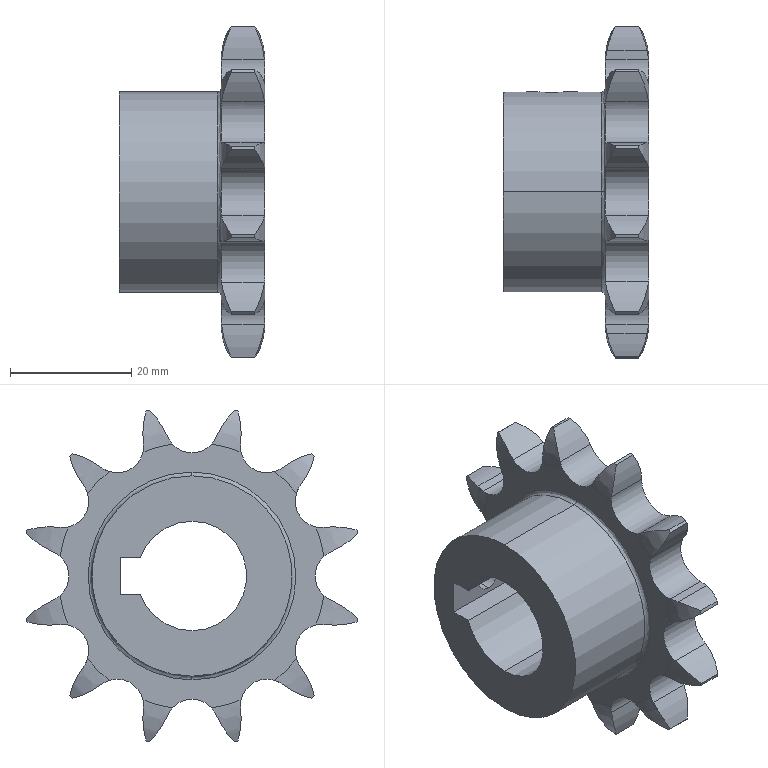Part | SolidWorks | features BaseBody 1, HoleWzd 1, ICE 1 | 1 solid | 94 faces | box 24.001 x 54.65 x 54.65 mm | volume 19561 mm3 | cylinder 62 | spline 26 | plane 6 | commonest cylinder face diameters 28.594 x26 8.595 x17 56.434 x12 18 x3 4.2 x2 33 x2